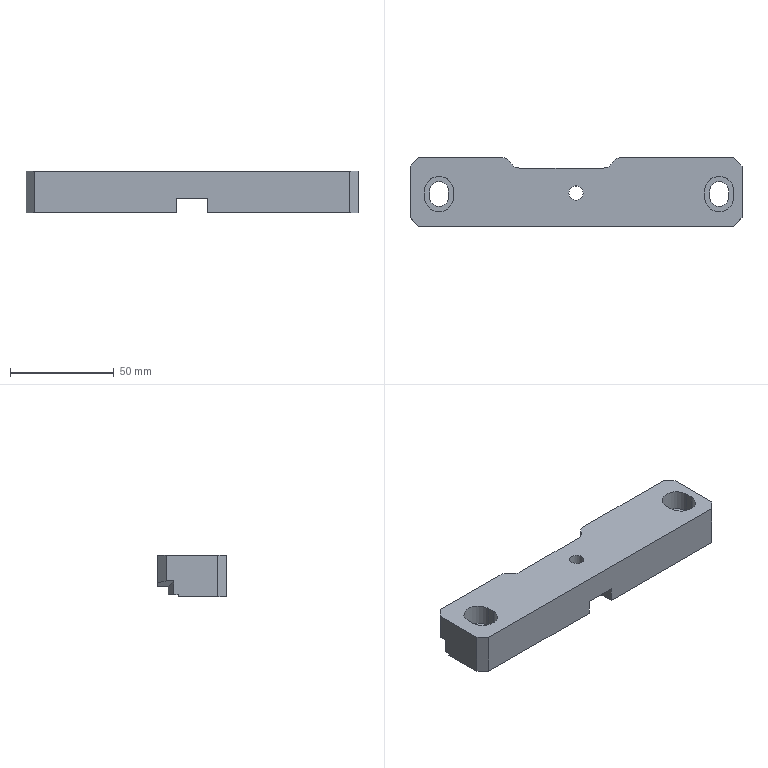Part | NX | features 20 2 | 1 solid | 49 faces | box 160 x 33 x 20 mm | volume 87274 mm3 | plane 36 | cylinder 13 | commonest cylinder face diameters 9 x4 10 x4 14 x4 6.8 x1
STEP:
#1=CARTESIAN_POINT('',(720.002,-433.5,16.5));
#2=VERTEX_POINT('',#1);
#3=CARTESIAN_POINT('',(720.002,-436.5,16.5));
#4=VERTEX_POINT('',#3);
#5=CARTESIAN_POINT('',(720.002,-450.5,16.5));
#6=DIRECTION('',(0.,-1.,0.));
#7=VECTOR('',#6,1000.);
#8=LINE('',#5,#7);
#9=EDGE_CURVE('',#2,#4,#8,.T.);
#10=ORIENTED_EDGE('',*,*,#9,.F.);
#11=CARTESIAN_POINT('',(734.002,-433.5,16.5));
#12=VERTEX_POINT('',#11);
#13=CARTESIAN_POINT('',(727.002,-433.5,16.5));
#14=DIRECTION('',(0.,0.,1.));
#15=DIRECTION('',(1.,0.,0.));
#16=AXIS2_PLACEMENT_3D('',#13,#14,#15);
#17=CIRCLE('',#16,7.);
#18=EDGE_CURVE('',#12,#2,#17,.T.);
#19=ORIENTED_EDGE('',*,*,#18,.F.);
#20=CARTESIAN_POINT('',(734.002,-436.5,16.5));
#21=VERTEX_POINT('',#20);
#22=CARTESIAN_POINT('',(734.002,-450.5,16.5));
#23=DIRECTION('',(0.,1.,0.));
#24=VECTOR('',#23,1000.);
#25=LINE('',#22,#24);
#26=EDGE_CURVE('',#21,#12,#25,.T.);
#27=ORIENTED_EDGE('',*,*,#26,.F.);
#28=CARTESIAN_POINT('',(727.002,-436.5,16.5));
#29=DIRECTION('',(0.,0.,1.));
#30=DIRECTION('',(1.,0.,0.));
#31=AXIS2_PLACEMENT_3D('',#28,#29,#30);
#32=CIRCLE('',#31,7.);
#33=EDGE_CURVE('',#4,#21,#32,.T.);
#34=ORIENTED_EDGE('',*,*,#33,.F.);
#35=EDGE_LOOP('',(#10,#19,#27,#34));
#36=FACE_BOUND('',#35,.T.);
#37=CARTESIAN_POINT('',(585.002,-433.5,16.5));
#38=VERTEX_POINT('',#37);
#39=CARTESIAN_POINT('',(585.002,-436.5,16.5));
#40=VERTEX_POINT('',#39);
#41=CARTESIAN_POINT('',(585.002,-450.5,16.5));
#42=DIRECTION('',(0.,-1.,0.));
#43=VECTOR('',#42,1000.);
#44=LINE('',#41,#43);
#45=EDGE_CURVE('',#38,#40,#44,.T.);
#46=ORIENTED_EDGE('',*,*,#45,.F.);
#47=CARTESIAN_POINT('',(599.002,-433.5,16.5));
#48=VERTEX_POINT('',#47);
#49=CARTESIAN_POINT('',(592.002,-433.5,16.5));
#50=DIRECTION('',(0.,0.,1.));
#51=DIRECTION('',(1.,0.,0.));
#52=AXIS2_PLACEMENT_3D('',#49,#50,#51);
#53=CIRCLE('',#52,7.);
#54=EDGE_CURVE('',#48,#38,#53,.T.);
#55=ORIENTED_EDGE('',*,*,#54,.F.);
#56=CARTESIAN_POINT('',(599.002,-436.5,16.5));
#57=VERTEX_POINT('',#56);
#58=CARTESIAN_POINT('',(599.002,-450.5,16.5));
#59=DIRECTION('',(0.,1.,0.));
#60=VECTOR('',#59,1000.);
#61=LINE('',#58,#60);
#62=EDGE_CURVE('',#57,#48,#61,.T.);
#63=ORIENTED_EDGE('',*,*,#62,.F.);
#64=CARTESIAN_POINT('',(592.002,-436.5,16.5));
#65=DIRECTION('',(0.,0.,1.));
#66=DIRECTION('',(1.,0.,0.));
#67=AXIS2_PLACEMENT_3D('',#64,#65,#66);
#68=CIRCLE('',#67,7.);
#69=EDGE_CURVE('',#40,#57,#68,.T.);
#70=ORIENTED_EDGE('',*,*,#69,.F.);
#71=EDGE_LOOP('',(#46,#55,#63,#70));
#72=FACE_BOUND('',#71,.T.);
#73=CARTESIAN_POINT('',(738.002,-446.5,16.5));
#74=VERTEX_POINT('',#73);
#75=CARTESIAN_POINT('',(738.002,-421.5,16.5));
#76=VERTEX_POINT('',#75);
#77=CARTESIAN_POINT('',(738.002,-450.5,16.5));
#78=DIRECTION('',(0.,1.,0.));
#79=VECTOR('',#78,1000.);
#80=LINE('',#77,#79);
#81=EDGE_CURVE('',#74,#76,#80,.T.);
#82=ORIENTED_EDGE('',*,*,#81,.T.);
#83=CARTESIAN_POINT('',(734.002,-417.5,16.5));
#84=VERTEX_POINT('',#83);
#85=CARTESIAN_POINT('',(734.002,-417.5,16.5));
#86=DIRECTION('',(-0.7071,0.7071,0.));
#87=VECTOR('',#86,1000.);
#88=LINE('',#85,#87);
#89=EDGE_CURVE('',#76,#84,#88,.T.);
#90=ORIENTED_EDGE('',*,*,#89,.T.);
#91=CARTESIAN_POINT('',(679.789,-417.5,16.5));
#92=VERTEX_POINT('',#91);
#93=CARTESIAN_POINT('',(766.002,-417.5,16.5));
#94=DIRECTION('',(-1.,0.,0.));
#95=VECTOR('',#94,1000.);
#96=LINE('',#93,#95);
#97=EDGE_CURVE('',#84,#92,#96,.T.);
#98=ORIENTED_EDGE('',*,*,#97,.T.);
#99=CARTESIAN_POINT('',(675.459,-420.,16.5));
#100=VERTEX_POINT('',#99);
#101=CARTESIAN_POINT('',(679.789,-422.5,16.5));
#102=DIRECTION('',(0.,0.,1.));
#103=DIRECTION('',(1.,0.,0.));
#104=AXIS2_PLACEMENT_3D('',#101,#102,#103);
#105=CIRCLE('',#104,5.);
#106=EDGE_CURVE('',#92,#100,#105,.T.);
#107=ORIENTED_EDGE('',*,*,#106,.T.);
#108=CARTESIAN_POINT('',(671.129,-422.5,16.5));
#109=VERTEX_POINT('',#108);
#110=CARTESIAN_POINT('',(671.129,-417.5,16.5));
#111=DIRECTION('',(0.,0.,1.));
#112=DIRECTION('',(1.,0.,0.));
#113=AXIS2_PLACEMENT_3D('',#110,#111,#112);
#114=CIRCLE('',#113,5.);
#115=EDGE_CURVE('',#109,#100,#114,.T.);
#116=ORIENTED_EDGE('',*,*,#115,.F.);
#117=CARTESIAN_POINT('',(630.929,-422.5,16.5));
#118=VERTEX_POINT('',#117);
#119=CARTESIAN_POINT('',(766.002,-422.5,16.5));
#120=DIRECTION('',(1.,0.,0.));
#121=VECTOR('',#120,1000.);
#122=LINE('',#119,#121);
#123=EDGE_CURVE('',#118,#109,#122,.T.);
#124=ORIENTED_EDGE('',*,*,#123,.F.);
#125=CARTESIAN_POINT('',(626.598,-420.,16.5));
#126=VERTEX_POINT('',#125);
#127=CARTESIAN_POINT('',(630.929,-417.5,16.5));
#128=DIRECTION('',(0.,0.,1.));
#129=DIRECTION('',(1.,0.,0.));
#130=AXIS2_PLACEMENT_3D('',#127,#128,#129);
#131=CIRCLE('',#130,5.);
#132=EDGE_CURVE('',#126,#118,#131,.T.);
#133=ORIENTED_EDGE('',*,*,#132,.F.);
#134=CARTESIAN_POINT('',(622.268,-417.5,16.5));
#135=VERTEX_POINT('',#134);
#136=CARTESIAN_POINT('',(622.268,-422.5,16.5));
#137=DIRECTION('',(0.,0.,1.));
#138=DIRECTION('',(1.,0.,0.));
#139=AXIS2_PLACEMENT_3D('',#136,#137,#138);
#140=CIRCLE('',#139,5.);
#141=EDGE_CURVE('',#126,#135,#140,.T.);
#142=ORIENTED_EDGE('',*,*,#141,.T.);
#143=CARTESIAN_POINT('',(582.002,-417.5,16.5));
#144=VERTEX_POINT('',#143);
#145=CARTESIAN_POINT('',(766.002,-417.5,16.5));
#146=DIRECTION('',(-1.,0.,0.));
#147=VECTOR('',#146,1000.);
#148=LINE('',#145,#147);
#149=EDGE_CURVE('',#135,#144,#148,.T.);
#150=ORIENTED_EDGE('',*,*,#149,.T.);
#151=CARTESIAN_POINT('',(578.002,-421.5,16.5));
#152=VERTEX_POINT('',#151);
#153=CARTESIAN_POINT('',(578.002,-421.5,16.5));
#154=DIRECTION('',(-0.7071,-0.7071,0.));
#155=VECTOR('',#154,1000.);
#156=LINE('',#153,#155);
#157=EDGE_CURVE('',#144,#152,#156,.T.);
#158=ORIENTED_EDGE('',*,*,#157,.T.);
#159=CARTESIAN_POINT('',(578.002,-446.5,16.5));
#160=VERTEX_POINT('',#159);
#161=CARTESIAN_POINT('',(578.002,-417.5,16.5));
#162=DIRECTION('',(0.,-1.,0.));
#163=VECTOR('',#162,1000.);
#164=LINE('',#161,#163);
#165=EDGE_CURVE('',#152,#160,#164,.T.);
#166=ORIENTED_EDGE('',*,*,#165,.T.);
#167=CARTESIAN_POINT('',(582.002,-450.5,16.5));
#168=VERTEX_POINT('',#167);
#169=CARTESIAN_POINT('',(582.002,-450.5,16.5));
#170=DIRECTION('',(0.7071,-0.7071,0.));
#171=VECTOR('',#170,1000.);
#172=LINE('',#169,#171);
#173=EDGE_CURVE('',#160,#168,#172,.T.);
#174=ORIENTED_EDGE('',*,*,#173,.T.);
#175=CARTESIAN_POINT('',(734.002,-450.5,16.5));
#176=VERTEX_POINT('',#175);
#177=CARTESIAN_POINT('',(686.002,-450.5,16.5));
#178=DIRECTION('',(1.,0.,0.));
#179=VECTOR('',#178,1000.);
#180=LINE('',#177,#179);
#181=EDGE_CURVE('',#168,#176,#180,.T.);
#182=ORIENTED_EDGE('',*,*,#181,.T.);
#183=CARTESIAN_POINT('',(738.002,-446.5,16.5));
#184=DIRECTION('',(0.7071,0.7071,0.));
#185=VECTOR('',#184,1000.);
#186=LINE('',#183,#185);
#187=EDGE_CURVE('',#176,#74,#186,.T.);
#188=ORIENTED_EDGE('',*,*,#187,.T.);
#189=EDGE_LOOP('',(#82,#90,#98,#107,#116,#124,#133,#142,#150,#158,#166,#174,#182,#188));
#190=FACE_BOUND('',#189,.T.);
#191=CARTESIAN_POINT('',(661.402,-434.5,16.5));
#192=VERTEX_POINT('',#191);
#193=CARTESIAN_POINT('',(658.002,-434.5,16.5));
#194=DIRECTION('',(0.,0.,-1.));
#195=DIRECTION('',(1.,0.,0.));
#196=AXIS2_PLACEMENT_3D('',#193,#194,#195);
#197=CIRCLE('',#196,3.4);
#198=EDGE_CURVE('',#192,#192,#197,.T.);
#199=ORIENTED_EDGE('',*,*,#198,.T.);
#200=EDGE_LOOP('',(#199));
#201=FACE_BOUND('',#200,.T.);
#202=CARTESIAN_POINT('',(766.002,-450.5,16.5));
#203=DIRECTION('',(0.,0.,1.));
#204=DIRECTION('',(-1.,0.,0.));
#205=AXIS2_PLACEMENT_3D('',#202,#203,#204);
#206=PLANE('',#205);
#207=ADVANCED_FACE('',(#36,#72,#190,#201),#206,.T.);
#208=CARTESIAN_POINT('',(630.929,-422.5,1.5));
#209=VERTEX_POINT('',#208);
#210=CARTESIAN_POINT('',(626.598,-420.,1.5));
#211=VERTEX_POINT('',#210);
#212=CARTESIAN_POINT('',(630.929,-417.5,1.5));
#213=DIRECTION('',(0.,0.,-1.));
#214=DIRECTION('',(-1.,0.,0.));
#215=AXIS2_PLACEMENT_3D('',#212,#213,#214);
#216=CIRCLE('',#215,5.);
#217=EDGE_CURVE('',#209,#211,#216,.T.);
#218=ORIENTED_EDGE('',*,*,#217,.F.);
#219=CARTESIAN_POINT('',(588.002,-422.5,1.5));
#220=VERTEX_POINT('',#219);
#221=CARTESIAN_POINT('',(704.001,-422.5,1.5));
#222=DIRECTION('',(1.,0.,0.));
#223=VECTOR('',#222,1000.);
#224=LINE('',#221,#223);
#225=EDGE_CURVE('',#220,#209,#224,.T.);
#226=ORIENTED_EDGE('',*,*,#225,.F.);
#227=CARTESIAN_POINT('',(588.002,-417.5,1.5));
#228=VERTEX_POINT('',#227);
#229=CARTESIAN_POINT('',(588.002,-417.5,1.5));
#230=DIRECTION('',(0.,1.,0.));
#231=VECTOR('',#230,1000.);
#232=LINE('',#229,#231);
#233=EDGE_CURVE('',#220,#228,#232,.T.);
#234=ORIENTED_EDGE('',*,*,#233,.T.);
#235=CARTESIAN_POINT('',(622.268,-417.5,1.5));
#236=VERTEX_POINT('',#235);
#237=CARTESIAN_POINT('',(714.002,-417.5,1.5));
#238=DIRECTION('',(1.,0.,0.));
#239=VECTOR('',#238,1000.);
#240=LINE('',#237,#239);
#241=EDGE_CURVE('',#228,#236,#240,.T.);
#242=ORIENTED_EDGE('',*,*,#241,.T.);
#243=CARTESIAN_POINT('',(622.268,-422.5,1.5));
#244=DIRECTION('',(0.,0.,-1.));
#245=DIRECTION('',(-1.,0.,0.));
#246=AXIS2_PLACEMENT_3D('',#243,#244,#245);
#247=CIRCLE('',#246,5.);
#248=EDGE_CURVE('',#236,#211,#247,.T.);
#249=ORIENTED_EDGE('',*,*,#248,.T.);
#250=EDGE_LOOP('',(#218,#226,#234,#242,#249));
#251=FACE_BOUND('',#250,.T.);
#252=CARTESIAN_POINT('',(736.273,-396.891,1.5));
#253=DIRECTION('',(0.,0.,-1.));
#254=DIRECTION('',(1.,0.,0.));
#255=AXIS2_PLACEMENT_3D('',#252,#253,#254);
#256=PLANE('',#255);
#257=ADVANCED_FACE('',(#251),#256,.T.);
#258=CARTESIAN_POINT('',(578.002,-427.372,-2.5));
#259=VERTEX_POINT('',#258);
#260=CARTESIAN_POINT('',(578.002,-427.372,-3.5));
#261=VERTEX_POINT('',#260);
#262=CARTESIAN_POINT('',(578.002,-427.372,11.5));
#263=DIRECTION('',(0.,0.,-1.));
#264=VECTOR('',#263,1000.);
#265=LINE('',#262,#264);
#266=EDGE_CURVE('',#259,#261,#265,.T.);
#267=ORIENTED_EDGE('',*,*,#266,.F.);
#268=CARTESIAN_POINT('',(609.502,-427.372,-2.5));
#269=VERTEX_POINT('',#268);
#270=CARTESIAN_POINT('',(684.583,-427.372,-2.5));
#271=DIRECTION('',(1.,0.,0.));
#272=VECTOR('',#271,1000.);
#273=LINE('',#270,#272);
#274=EDGE_CURVE('',#259,#269,#273,.T.);
#275=ORIENTED_EDGE('',*,*,#274,.T.);
#276=CARTESIAN_POINT('',(650.502,-427.372,-2.5));
#277=VERTEX_POINT('',#276);
#278=CARTESIAN_POINT('',(630.002,-427.372,-2.5));
#279=DIRECTION('',(1.,0.,0.));
#280=VECTOR('',#279,1000.);
#281=LINE('',#278,#280);
#282=EDGE_CURVE('',#269,#277,#281,.T.);
#283=ORIENTED_EDGE('',*,*,#282,.T.);
#284=CARTESIAN_POINT('',(650.502,-427.372,-3.5));
#285=VERTEX_POINT('',#284);
#286=CARTESIAN_POINT('',(650.502,-427.372,-9.5));
#287=DIRECTION('',(0.,0.,-1.));
#288=VECTOR('',#287,1000.);
#289=LINE('',#286,#288);
#290=EDGE_CURVE('',#277,#285,#289,.T.);
#291=ORIENTED_EDGE('',*,*,#290,.T.);
#292=CARTESIAN_POINT('',(766.002,-427.372,-3.5));
#293=DIRECTION('',(-1.,0.,0.));
#294=VECTOR('',#293,1000.);
#295=LINE('',#292,#294);
#296=EDGE_CURVE('',#285,#261,#295,.T.);
#297=ORIENTED_EDGE('',*,*,#296,.T.);
#298=EDGE_LOOP('',(#267,#275,#283,#291,#297));
#299=FACE_BOUND('',#298,.T.);
#300=CARTESIAN_POINT('',(684.583,-427.372,-21.));
#301=DIRECTION('',(0.,1.,0.));
#302=DIRECTION('',(0.,0.,-1.));
#303=AXIS2_PLACEMENT_3D('',#300,#301,#302);
#304=PLANE('',#303);
#305=ADVANCED_FACE('',(#299),#304,.T.);
#306=CARTESIAN_POINT('',(665.502,-427.372,-2.5));
#307=VERTEX_POINT('',#306);
#308=CARTESIAN_POINT('',(665.502,-427.372,-3.5));
#309=VERTEX_POINT('',#308);
#310=CARTESIAN_POINT('',(665.502,-427.372,-9.5));
#311=DIRECTION('',(0.,0.,-1.));
#312=VECTOR('',#311,1000.);
#313=LINE('',#310,#312);
#314=EDGE_CURVE('',#307,#309,#313,.T.);
#315=ORIENTED_EDGE('',*,*,#314,.F.);
#316=CARTESIAN_POINT('',(738.002,-427.372,-2.5));
#317=VERTEX_POINT('',#316);
#318=CARTESIAN_POINT('',(684.583,-427.372,-2.5));
#319=DIRECTION('',(1.,0.,0.));
#320=VECTOR('',#319,1000.);
#321=LINE('',#318,#320);
#322=EDGE_CURVE('',#307,#317,#321,.T.);
#323=ORIENTED_EDGE('',*,*,#322,.T.);
#324=CARTESIAN_POINT('',(738.002,-427.372,-3.5));
#325=VERTEX_POINT('',#324);
#326=CARTESIAN_POINT('',(738.002,-427.372,11.5));
#327=DIRECTION('',(0.,0.,1.));
#328=VECTOR('',#327,1000.);
#329=LINE('',#326,#328);
#330=EDGE_CURVE('',#325,#317,#329,.T.);
#331=ORIENTED_EDGE('',*,*,#330,.F.);
#332=CARTESIAN_POINT('',(646.002,-427.372,-3.5));
#333=DIRECTION('',(-1.,0.,0.));
#334=VECTOR('',#333,1000.);
#335=LINE('',#332,#334);
#336=EDGE_CURVE('',#325,#309,#335,.T.);
#337=ORIENTED_EDGE('',*,*,#336,.T.);
#338=EDGE_LOOP('',(#315,#323,#331,#337));
#339=FACE_BOUND('',#338,.T.);
#340=CARTESIAN_POINT('',(684.583,-427.372,-21.));
#341=DIRECTION('',(0.,1.,0.));
#342=DIRECTION('',(0.,0.,-1.));
#343=AXIS2_PLACEMENT_3D('',#340,#341,#342);
#344=PLANE('',#343);
#345=ADVANCED_FACE('',(#339),#344,.T.);
#346=CARTESIAN_POINT('',(738.002,-446.5,-3.5));
#347=VERTEX_POINT('',#346);
#348=CARTESIAN_POINT('',(734.002,-450.5,-3.5));
#349=VERTEX_POINT('',#348);
#350=CARTESIAN_POINT('',(738.002,-446.5,-3.5));
#351=DIRECTION('',(-0.7071,-0.7071,0.));
#352=VECTOR('',#351,1000.);
#353=LINE('',#350,#352);
#354=EDGE_CURVE('',#347,#349,#353,.T.);
#355=ORIENTED_EDGE('',*,*,#354,.F.);
#356=CARTESIAN_POINT('',(738.002,-446.5,11.5));
#357=DIRECTION('',(0.,0.,-1.));
#358=VECTOR('',#357,1000.);
#359=LINE('',#356,#358);
#360=EDGE_CURVE('',#74,#347,#359,.T.);
#361=ORIENTED_EDGE('',*,*,#360,.F.);
#362=ORIENTED_EDGE('',*,*,#187,.F.);
#363=CARTESIAN_POINT('',(734.002,-450.5,11.5));
#364=DIRECTION('',(0.,0.,1.));
#365=VECTOR('',#364,1000.);
#366=LINE('',#363,#365);
#367=EDGE_CURVE('',#349,#176,#366,.T.);
#368=ORIENTED_EDGE('',*,*,#367,.F.);
#369=EDGE_LOOP('',(#355,#361,#362,#368));
#370=FACE_BOUND('',#369,.T.);
#371=CARTESIAN_POINT('',(738.002,-446.5,11.5));
#372=DIRECTION('',(-0.7071,0.7071,0.));
#373=DIRECTION('',(0.,0.,-1.));
#374=AXIS2_PLACEMENT_3D('',#371,#372,#373);
#375=PLANE('',#374);
#376=ADVANCED_FACE('',(#370),#375,.F.);
#377=CARTESIAN_POINT('',(582.002,-450.5,-3.5));
#378=VERTEX_POINT('',#377);
#379=CARTESIAN_POINT('',(578.002,-446.5,-3.5));
#380=VERTEX_POINT('',#379);
#381=CARTESIAN_POINT('',(582.002,-450.5,-3.5));
#382=DIRECTION('',(-0.7071,0.7071,0.));
#383=VECTOR('',#382,1000.);
#384=LINE('',#381,#383);
#385=EDGE_CURVE('',#378,#380,#384,.T.);
#386=ORIENTED_EDGE('',*,*,#385,.F.);
#387=CARTESIAN_POINT('',(582.002,-450.5,11.5));
#388=DIRECTION('',(0.,0.,-1.));
#389=VECTOR('',#388,1000.);
#390=LINE('',#387,#389);
#391=EDGE_CURVE('',#168,#378,#390,.T.);
#392=ORIENTED_EDGE('',*,*,#391,.F.);
#393=ORIENTED_EDGE('',*,*,#173,.F.);
#394=CARTESIAN_POINT('',(578.002,-446.5,11.5));
#395=DIRECTION('',(0.,0.,1.));
#396=VECTOR('',#395,1000.);
#397=LINE('',#394,#396);
#398=EDGE_CURVE('',#380,#160,#397,.T.);
#399=ORIENTED_EDGE('',*,*,#398,.F.);
#400=EDGE_LOOP('',(#386,#392,#393,#399));
#401=FACE_BOUND('',#400,.T.);
#402=CARTESIAN_POINT('',(582.002,-450.5,11.5));
#403=DIRECTION('',(0.7071,0.7071,0.));
#404=DIRECTION('',(0.,0.,-1.));
#405=AXIS2_PLACEMENT_3D('',#402,#403,#404);
#406=PLANE('',#405);
#407=ADVANCED_FACE('',(#401),#406,.F.);
#408=ORIENTED_EDGE('',*,*,#33,.T.);
#409=CARTESIAN_POINT('',(734.002,-436.5,6.5));
#410=VERTEX_POINT('',#409);
#411=CARTESIAN_POINT('',(734.002,-436.5,42.5));
#412=DIRECTION('',(0.,0.,1.));
#413=VECTOR('',#412,1000.);
#414=LINE('',#411,#413);
#415=EDGE_CURVE('',#410,#21,#414,.T.);
#416=ORIENTED_EDGE('',*,*,#415,.F.);
#417=CARTESIAN_POINT('',(720.002,-436.5,6.5));
#418=VERTEX_POINT('',#417);
#419=CARTESIAN_POINT('',(727.002,-436.5,6.5));
#420=DIRECTION('',(0.,0.,1.));
#421=DIRECTION('',(-1.,0.,0.));
#422=AXIS2_PLACEMENT_3D('',#419,#420,#421);
#423=CIRCLE('',#422,7.);
#424=EDGE_CURVE('',#418,#410,#423,.T.);
#425=ORIENTED_EDGE('',*,*,#424,.F.);
#426=CARTESIAN_POINT('',(720.002,-436.5,42.5));
#427=DIRECTION('',(0.,0.,1.));
#428=VECTOR('',#427,1000.);
#429=LINE('',#426,#428);
#430=EDGE_CURVE('',#418,#4,#429,.T.);
#431=ORIENTED_EDGE('',*,*,#430,.T.);
#432=EDGE_LOOP('',(#408,#416,#425,#431));
#433=FACE_BOUND('',#432,.T.);
#434=CARTESIAN_POINT('',(727.002,-436.5,42.5));
#435=DIRECTION('',(0.,0.,-1.));
#436=DIRECTION('',(1.,0.,0.));
#437=AXIS2_PLACEMENT_3D('',#434,#435,#436);
#438=CYLINDRICAL_SURFACE('',#437,7.);
#439=ADVANCED_FACE('',(#433),#438,.F.);
#440=CARTESIAN_POINT('',(731.502,-436.5,6.5));
#441=VERTEX_POINT('',#440);
#442=CARTESIAN_POINT('',(722.502,-436.5,6.5));
#443=VERTEX_POINT('',#442);
#444=CARTESIAN_POINT('',(727.002,-436.5,6.5));
#445=DIRECTION('',(0.,0.,-1.));
#446=DIRECTION('',(-1.,0.,0.));
#447=AXIS2_PLACEMENT_3D('',#444,#445,#446);
#448=CIRCLE('',#447,4.5);
#449=EDGE_CURVE('',#441,#443,#448,.T.);
#450=ORIENTED_EDGE('',*,*,#449,.F.);
#451=CARTESIAN_POINT('',(731.502,-436.5,-3.5));
#452=VERTEX_POINT('',#451);
#453=CARTESIAN_POINT('',(731.502,-436.5,42.5));
#454=DIRECTION('',(0.,0.,1.));
#455=VECTOR('',#454,1000.);
#456=LINE('',#453,#455);
#457=EDGE_CURVE('',#452,#441,#456,.T.);
#458=ORIENTED_EDGE('',*,*,#457,.F.);
#459=CARTESIAN_POINT('',(722.502,-436.5,-3.5));
#460=VERTEX_POINT('',#459);
#461=CARTESIAN_POINT('',(727.002,-436.5,-3.5));
#462=DIRECTION('',(0.,0.,1.));
#463=DIRECTION('',(1.,0.,0.));
#464=AXIS2_PLACEMENT_3D('',#461,#462,#463);
#465=CIRCLE('',#464,4.5);
#466=EDGE_CURVE('',#460,#452,#465,.T.);
#467=ORIENTED_EDGE('',*,*,#466,.F.);
#468=CARTESIAN_POINT('',(722.502,-436.5,42.5));
#469=DIRECTION('',(0.,0.,1.));
#470=VECTOR('',#469,1000.);
#471=LINE('',#468,#470);
#472=EDGE_CURVE('',#460,#443,#471,.T.);
#473=ORIENTED_EDGE('',*,*,#472,.T.);
#474=EDGE_LOOP('',(#450,#458,#467,#473));
#475=FACE_BOUND('',#474,.T.);
#476=CARTESIAN_POINT('',(727.002,-436.5,42.5));
#477=DIRECTION('',(0.,0.,-1.));
#478=DIRECTION('',(1.,0.,0.));
#479=AXIS2_PLACEMENT_3D('',#476,#477,#478);
#480=CYLINDRICAL_SURFACE('',#479,4.5);
#481=ADVANCED_FACE('',(#475),#480,.F.);
#482=CARTESIAN_POINT('',(731.502,-433.5,6.5));
#483=VERTEX_POINT('',#482);
#484=CARTESIAN_POINT('',(731.502,-439.5,6.5));
#485=DIRECTION('',(0.,-1.,0.));
#486=VECTOR('',#485,1000.);
#487=LINE('',#484,#486);
#488=EDGE_CURVE('',#483,#441,#487,.T.);
#489=ORIENTED_EDGE('',*,*,#488,.F.);
#490=CARTESIAN_POINT('',(731.502,-433.5,-3.5));
#491=VERTEX_POINT('',#490);
#492=CARTESIAN_POINT('',(731.502,-433.5,42.5));
#493=DIRECTION('',(0.,0.,1.));
#494=VECTOR('',#493,1000.);
#495=LINE('',#492,#494);
#496=EDGE_CURVE('',#491,#483,#495,.T.);
#497=ORIENTED_EDGE('',*,*,#496,.F.);
#498=CARTESIAN_POINT('',(731.502,-439.5,-3.5));
#499=DIRECTION('',(0.,1.,0.));
#500=VECTOR('',#499,1000.);
#501=LINE('',#498,#500);
#502=EDGE_CURVE('',#452,#491,#501,.T.);
#503=ORIENTED_EDGE('',*,*,#502,.F.);
#504=ORIENTED_EDGE('',*,*,#457,.T.);
#505=EDGE_LOOP('',(#489,#497,#503,#504));
#506=FACE_BOUND('',#505,.T.);
#507=CARTESIAN_POINT('',(731.502,-439.5,42.5));
#508=DIRECTION('',(-1.,0.,0.));
#509=DIRECTION('',(0.,0.,-1.));
#510=AXIS2_PLACEMENT_3D('',#507,#508,#509);
#511=PLANE('',#510);
#512=ADVANCED_FACE('',(#506),#511,.T.);
#513=CARTESIAN_POINT('',(722.502,-433.5,6.5));
#514=VERTEX_POINT('',#513);
#515=CARTESIAN_POINT('',(727.002,-433.5,6.5));
#516=DIRECTION('',(0.,0.,-1.));
#517=DIRECTION('',(-1.,0.,0.));
#518=AXIS2_PLACEMENT_3D('',#515,#516,#517);
#519=CIRCLE('',#518,4.5);
#520=EDGE_CURVE('',#514,#483,#519,.T.);
#521=ORIENTED_EDGE('',*,*,#520,.F.);
#522=CARTESIAN_POINT('',(722.502,-433.5,-3.5));
#523=VERTEX_POINT('',#522);
#524=CARTESIAN_POINT('',(722.502,-433.5,42.5));
#525=DIRECTION('',(0.,0.,1.));
#526=VECTOR('',#525,1000.);
#527=LINE('',#524,#526);
#528=EDGE_CURVE('',#523,#514,#527,.T.);
#529=ORIENTED_EDGE('',*,*,#528,.F.);
#530=CARTESIAN_POINT('',(727.002,-433.5,-3.5));
#531=DIRECTION('',(0.,0.,1.));
#532=DIRECTION('',(1.,0.,0.));
#533=AXIS2_PLACEMENT_3D('',#530,#531,#532);
#534=CIRCLE('',#533,4.5);
#535=EDGE_CURVE('',#491,#523,#534,.T.);
#536=ORIENTED_EDGE('',*,*,#535,.F.);
#537=ORIENTED_EDGE('',*,*,#496,.T.);
#538=EDGE_LOOP('',(#521,#529,#536,#537));
#539=FACE_BOUND('',#538,.T.);
#540=CARTESIAN_POINT('',(727.002,-433.5,42.5));
#541=DIRECTION('',(0.,0.,-1.));
#542=DIRECTION('',(1.,0.,0.));
#543=AXIS2_PLACEMENT_3D('',#540,#541,#542);
#544=CYLINDRICAL_SURFACE('',#543,4.5);
#545=ADVANCED_FACE('',(#539),#544,.F.);
#546=CARTESIAN_POINT('',(722.502,-432.5,6.5));
#547=DIRECTION('',(0.,1.,0.));
#548=VECTOR('',#547,1000.);
#549=LINE('',#546,#548);
#550=EDGE_CURVE('',#443,#514,#549,.T.);
#551=ORIENTED_EDGE('',*,*,#550,.F.);
#552=ORIENTED_EDGE('',*,*,#472,.F.);
#553=CARTESIAN_POINT('',(722.502,-432.5,-3.5));
#554=DIRECTION('',(0.,-1.,0.));
#555=VECTOR('',#554,1000.);
#556=LINE('',#553,#555);
#557=EDGE_CURVE('',#523,#460,#556,.T.);
#558=ORIENTED_EDGE('',*,*,#557,.F.);
#559=ORIENTED_EDGE('',*,*,#528,.T.);
#560=EDGE_LOOP('',(#551,#552,#558,#559));
#561=FACE_BOUND('',#560,.T.);
#562=CARTESIAN_POINT('',(722.502,-432.5,42.5));
#563=DIRECTION('',(1.,0.,0.));
#564=DIRECTION('',(0.,0.,1.));
#565=AXIS2_PLACEMENT_3D('',#562,#563,#564);
#566=PLANE('',#565);
#567=ADVANCED_FACE('',(#561),#566,.T.);
#568=ORIENTED_EDGE('',*,*,#69,.T.);
#569=CARTESIAN_POINT('',(599.002,-436.5,6.5));
#570=VERTEX_POINT('',#569);
#571=CARTESIAN_POINT('',(599.002,-436.5,42.5));
#572=DIRECTION('',(0.,0.,-1.));
#573=VECTOR('',#572,1000.);
#574=LINE('',#571,#573);
#575=EDGE_CURVE('',#57,#570,#574,.T.);
#576=ORIENTED_EDGE('',*,*,#575,.T.);
#577=CARTESIAN_POINT('',(585.002,-436.5,6.5));
#578=VERTEX_POINT('',#577);
#579=CARTESIAN_POINT('',(592.002,-436.5,6.5));
#580=DIRECTION('',(0.,0.,1.));
#581=DIRECTION('',(-1.,0.,0.));
#582=AXIS2_PLACEMENT_3D('',#579,#580,#581);
#583=CIRCLE('',#582,7.);
#584=EDGE_CURVE('',#578,#570,#583,.T.);
#585=ORIENTED_EDGE('',*,*,#584,.F.);
#586=CARTESIAN_POINT('',(585.002,-436.5,42.5));
#587=DIRECTION('',(0.,0.,-1.));
#588=VECTOR('',#587,1000.);
#589=LINE('',#586,#588);
#590=EDGE_CURVE('',#40,#578,#589,.T.);
#591=ORIENTED_EDGE('',*,*,#590,.F.);
#592=EDGE_LOOP('',(#568,#576,#585,#591));
#593=FACE_BOUND('',#592,.T.);
#594=CARTESIAN_POINT('',(592.002,-436.5,42.5));
#595=DIRECTION('',(0.,0.,-1.));
#596=DIRECTION('',(-1.,0.,0.));
#597=AXIS2_PLACEMENT_3D('',#594,#595,#596);
#598=CYLINDRICAL_SURFACE('',#597,7.);
#599=ADVANCED_FACE('',(#593),#598,.F.);
#600=CARTESIAN_POINT('',(587.502,-433.5,6.5));
#601=VERTEX_POINT('',#600);
#602=CARTESIAN_POINT('',(596.502,-433.5,6.5));
#603=VERTEX_POINT('',#602);
#604=CARTESIAN_POINT('',(592.002,-433.5,6.5));
#605=DIRECTION('',(0.,0.,-1.));
#606=DIRECTION('',(-1.,0.,0.));
#607=AXIS2_PLACEMENT_3D('',#604,#605,#606);
#608=CIRCLE('',#607,4.5);
#609=EDGE_CURVE('',#601,#603,#608,.T.);
#610=ORIENTED_EDGE('',*,*,#609,.F.);
#611=CARTESIAN_POINT('',(587.502,-433.5,-3.5));
#612=VERTEX_POINT('',#611);
#613=CARTESIAN_POINT('',(587.502,-433.5,42.5));
#614=DIRECTION('',(0.,0.,-1.));
#615=VECTOR('',#614,1000.);
#616=LINE('',#613,#615);
#617=EDGE_CURVE('',#601,#612,#616,.T.);
#618=ORIENTED_EDGE('',*,*,#617,.T.);
#619=CARTESIAN_POINT('',(596.502,-433.5,-3.5));
#620=VERTEX_POINT('',#619);
#621=CARTESIAN_POINT('',(592.002,-433.5,-3.5));
#622=DIRECTION('',(0.,0.,-1.));
#623=DIRECTION('',(1.,0.,0.));
#624=AXIS2_PLACEMENT_3D('',#621,#622,#623);
#625=CIRCLE('',#624,4.5);
#626=EDGE_CURVE('',#612,#620,#625,.T.);
#627=ORIENTED_EDGE('',*,*,#626,.T.);
#628=CARTESIAN_POINT('',(596.502,-433.5,42.5));
#629=DIRECTION('',(0.,0.,-1.));
#630=VECTOR('',#629,1000.);
#631=LINE('',#628,#630);
#632=EDGE_CURVE('',#603,#620,#631,.T.);
#633=ORIENTED_EDGE('',*,*,#632,.F.);
#634=EDGE_LOOP('',(#610,#618,#627,#633));
#635=FACE_BOUND('',#634,.T.);
#636=CARTESIAN_POINT('',(592.002,-433.5,42.5));
#637=DIRECTION('',(0.,0.,-1.));
#638=DIRECTION('',(-1.,0.,0.));
#639=AXIS2_PLACEMENT_3D('',#636,#637,#638);
#640=CYLINDRICAL_SURFACE('',#639,4.5);
#641=ADVANCED_FACE('',(#635),#640,.F.);
#642=CARTESIAN_POINT('',(587.502,-436.5,6.5));
#643=VERTEX_POINT('',#642);
#644=CARTESIAN_POINT('',(587.502,-439.5,6.5));
#645=DIRECTION('',(0.,1.,0.));
#646=VECTOR('',#645,1000.);
#647=LINE('',#644,#646);
#648=EDGE_CURVE('',#643,#601,#647,.T.);
#649=ORIENTED_EDGE('',*,*,#648,.F.);
#650=CARTESIAN_POINT('',(587.502,-436.5,-3.5));
#651=VERTEX_POINT('',#650);
#652=CARTESIAN_POINT('',(587.502,-436.5,42.5));
#653=DIRECTION('',(0.,0.,-1.));
#654=VECTOR('',#653,1000.);
#655=LINE('',#652,#654);
#656=EDGE_CURVE('',#643,#651,#655,.T.);
#657=ORIENTED_EDGE('',*,*,#656,.T.);
#658=CARTESIAN_POINT('',(587.502,-450.5,-3.5));
#659=DIRECTION('',(0.,1.,0.));
#660=VECTOR('',#659,1000.);
#661=LINE('',#658,#660);
#662=EDGE_CURVE('',#651,#612,#661,.T.);
#663=ORIENTED_EDGE('',*,*,#662,.T.);
#664=ORIENTED_EDGE('',*,*,#617,.F.);
#665=EDGE_LOOP('',(#649,#657,#663,#664));
#666=FACE_BOUND('',#665,.T.);
#667=CARTESIAN_POINT('',(587.502,-439.5,42.5));
#668=DIRECTION('',(1.,0.,0.));
#669=DIRECTION('',(0.,0.,-1.));
#670=AXIS2_PLACEMENT_3D('',#667,#668,#669);
#671=PLANE('',#670);
#672=ADVANCED_FACE('',(#666),#671,.T.);
#673=CARTESIAN_POINT('',(596.502,-436.5,6.5));
#674=VERTEX_POINT('',#673);
#675=CARTESIAN_POINT('',(592.002,-436.5,6.5));
#676=DIRECTION('',(0.,0.,-1.));
#677=DIRECTION('',(-1.,0.,0.));
#678=AXIS2_PLACEMENT_3D('',#675,#676,#677);
#679=CIRCLE('',#678,4.5);
#680=EDGE_CURVE('',#674,#643,#679,.T.);
#681=ORIENTED_EDGE('',*,*,#680,.F.);
#682=CARTESIAN_POINT('',(596.502,-436.5,-3.5));
#683=VERTEX_POINT('',#682);
#684=CARTESIAN_POINT('',(596.502,-436.5,42.5));
#685=DIRECTION('',(0.,0.,-1.));
#686=VECTOR('',#685,1000.);
#687=LINE('',#684,#686);
#688=EDGE_CURVE('',#674,#683,#687,.T.);
#689=ORIENTED_EDGE('',*,*,#688,.T.);
#690=CARTESIAN_POINT('',(592.002,-436.5,-3.5));
#691=DIRECTION('',(0.,0.,-1.));
#692=DIRECTION('',(1.,0.,0.));
#693=AXIS2_PLACEMENT_3D('',#690,#691,#692);
#694=CIRCLE('',#693,4.5);
#695=EDGE_CURVE('',#683,#651,#694,.T.);
#696=ORIENTED_EDGE('',*,*,#695,.T.);
#697=ORIENTED_EDGE('',*,*,#656,.F.);
#698=EDGE_LOOP('',(#681,#689,#696,#697));
#699=FACE_BOUND('',#698,.T.);
#700=CARTESIAN_POINT('',(592.002,-436.5,42.5));
#701=DIRECTION('',(0.,0.,-1.));
#702=DIRECTION('',(-1.,0.,0.));
#703=AXIS2_PLACEMENT_3D('',#700,#701,#702);
#704=CYLINDRICAL_SURFACE('',#703,4.5);
#705=ADVANCED_FACE('',(#699),#704,.F.);
#706=CARTESIAN_POINT('',(596.502,-432.5,6.5));
#707=DIRECTION('',(0.,-1.,0.));
#708=VECTOR('',#707,1000.);
#709=LINE('',#706,#708);
#710=EDGE_CURVE('',#603,#674,#709,.T.);
#711=ORIENTED_EDGE('',*,*,#710,.F.);
#712=ORIENTED_EDGE('',*,*,#632,.T.);
#713=CARTESIAN_POINT('',(596.502,-450.5,-3.5));
#714=DIRECTION('',(0.,-1.,0.));
#715=VECTOR('',#714,1000.);
#716=LINE('',#713,#715);
#717=EDGE_CURVE('',#620,#683,#716,.T.);
#718=ORIENTED_EDGE('',*,*,#717,.T.);
#719=ORIENTED_EDGE('',*,*,#688,.F.);
#720=EDGE_LOOP('',(#711,#712,#718,#719));
#721=FACE_BOUND('',#720,.T.);
#722=CARTESIAN_POINT('',(596.502,-432.5,42.5));
#723=DIRECTION('',(-1.,0.,0.));
#724=DIRECTION('',(0.,0.,1.));
#725=AXIS2_PLACEMENT_3D('',#722,#723,#724);
#726=PLANE('',#725);
#727=ADVANCED_FACE('',(#721),#726,.T.);
#728=ORIENTED_EDGE('',*,*,#26,.T.);
#729=CARTESIAN_POINT('',(734.002,-433.5,6.5));
#730=VERTEX_POINT('',#729);
#731=CARTESIAN_POINT('',(734.002,-433.5,42.5));
#732=DIRECTION('',(0.,0.,1.));
#733=VECTOR('',#732,1000.);
#734=LINE('',#731,#733);
#735=EDGE_CURVE('',#730,#12,#734,.T.);
#736=ORIENTED_EDGE('',*,*,#735,.F.);
#737=CARTESIAN_POINT('',(734.002,-432.5,6.5));
#738=DIRECTION('',(0.,1.,0.));
#739=VECTOR('',#738,1000.);
#740=LINE('',#737,#739);
#741=EDGE_CURVE('',#410,#730,#740,.T.);
#742=ORIENTED_EDGE('',*,*,#741,.F.);
#743=ORIENTED_EDGE('',*,*,#415,.T.);
#744=EDGE_LOOP('',(#728,#736,#742,#743));
#745=FACE_BOUND('',#744,.T.);
#746=CARTESIAN_POINT('',(734.002,-432.5,42.5));
#747=DIRECTION('',(1.,0.,0.));
#748=DIRECTION('',(0.,0.,1.));
#749=AXIS2_PLACEMENT_3D('',#746,#747,#748);
#750=PLANE('',#749);
#751=ADVANCED_FACE('',(#745),#750,.F.);
#752=ORIENTED_EDGE('',*,*,#9,.T.);
#753=ORIENTED_EDGE('',*,*,#430,.F.);
#754=CARTESIAN_POINT('',(720.002,-433.5,6.5));
#755=VERTEX_POINT('',#754);
#756=CARTESIAN_POINT('',(720.002,-439.5,6.5));
#757=DIRECTION('',(0.,-1.,0.));
#758=VECTOR('',#757,1000.);
#759=LINE('',#756,#758);
#760=EDGE_CURVE('',#755,#418,#759,.T.);
#761=ORIENTED_EDGE('',*,*,#760,.F.);
#762=CARTESIAN_POINT('',(720.002,-433.5,42.5));
#763=DIRECTION('',(0.,0.,1.));
#764=VECTOR('',#763,1000.);
#765=LINE('',#762,#764);
#766=EDGE_CURVE('',#755,#2,#765,.T.);
#767=ORIENTED_EDGE('',*,*,#766,.T.);
#768=EDGE_LOOP('',(#752,#753,#761,#767));
#769=FACE_BOUND('',#768,.T.);
#770=CARTESIAN_POINT('',(720.002,-439.5,42.5));
#771=DIRECTION('',(-1.,0.,0.));
#772=DIRECTION('',(0.,0.,-1.));
#773=AXIS2_PLACEMENT_3D('',#770,#771,#772);
#774=PLANE('',#773);
#775=ADVANCED_FACE('',(#769),#774,.F.);
#776=ORIENTED_EDGE('',*,*,#62,.T.);
#777=CARTESIAN_POINT('',(599.002,-433.5,6.5));
#778=VERTEX_POINT('',#777);
#779=CARTESIAN_POINT('',(599.002,-433.5,42.5));
#780=DIRECTION('',(0.,0.,-1.));
#781=VECTOR('',#780,1000.);
#782=LINE('',#779,#781);
#783=EDGE_CURVE('',#48,#778,#782,.T.);
#784=ORIENTED_EDGE('',*,*,#783,.T.);
#785=CARTESIAN_POINT('',(599.002,-439.5,6.5));
#786=DIRECTION('',(0.,1.,0.));
#787=VECTOR('',#786,1000.);
#788=LINE('',#785,#787);
#789=EDGE_CURVE('',#570,#778,#788,.T.);
#790=ORIENTED_EDGE('',*,*,#789,.F.);
#791=ORIENTED_EDGE('',*,*,#575,.F.);
#792=EDGE_LOOP('',(#776,#784,#790,#791));
#793=FACE_BOUND('',#792,.T.);
#794=CARTESIAN_POINT('',(599.002,-439.5,42.5));
#795=DIRECTION('',(1.,0.,0.));
#796=DIRECTION('',(0.,0.,-1.));
#797=AXIS2_PLACEMENT_3D('',#794,#795,#796);
#798=PLANE('',#797);
#799=ADVANCED_FACE('',(#793),#798,.F.);
#800=ORIENTED_EDGE('',*,*,#45,.T.);
#801=ORIENTED_EDGE('',*,*,#590,.T.);
#802=CARTESIAN_POINT('',(585.002,-433.5,6.5));
#803=VERTEX_POINT('',#802);
#804=CARTESIAN_POINT('',(585.002,-432.5,6.5));
#805=DIRECTION('',(0.,-1.,0.));
#806=VECTOR('',#805,1000.);
#807=LINE('',#804,#806);
#808=EDGE_CURVE('',#803,#578,#807,.T.);
#809=ORIENTED_EDGE('',*,*,#808,.F.);
#810=CARTESIAN_POINT('',(585.002,-433.5,42.5));
#811=DIRECTION('',(0.,0.,-1.));
#812=VECTOR('',#811,1000.);
#813=LINE('',#810,#812);
#814=EDGE_CURVE('',#38,#803,#813,.T.);
#815=ORIENTED_EDGE('',*,*,#814,.F.);
#816=EDGE_LOOP('',(#800,#801,#809,#815));
#817=FACE_BOUND('',#816,.T.);
#818=CARTESIAN_POINT('',(585.002,-432.5,42.5));
#819=DIRECTION('',(-1.,0.,0.));
#820=DIRECTION('',(0.,0.,1.));
#821=AXIS2_PLACEMENT_3D('',#818,#819,#820);
#822=PLANE('',#821);
#823=ADVANCED_FACE('',(#817),#822,.F.);
#824=CARTESIAN_POINT('',(650.502,-450.5,-3.5));
#825=VERTEX_POINT('',#824);
#826=CARTESIAN_POINT('',(650.502,-450.5,3.5));
#827=VERTEX_POINT('',#826);
#828=CARTESIAN_POINT('',(650.502,-450.5,11.5));
#829=DIRECTION('',(0.,0.,1.));
#830=VECTOR('',#829,1000.);
#831=LINE('',#828,#830);
#832=EDGE_CURVE('',#825,#827,#831,.T.);
#833=ORIENTED_EDGE('',*,*,#832,.T.);
#834=CARTESIAN_POINT('',(665.502,-450.5,3.5));
#835=VERTEX_POINT('',#834);
#836=CARTESIAN_POINT('',(686.002,-450.5,3.5));
#837=DIRECTION('',(1.,0.,0.));
#838=VECTOR('',#837,1000.);
#839=LINE('',#836,#838);
#840=EDGE_CURVE('',#827,#835,#839,.T.);
#841=ORIENTED_EDGE('',*,*,#840,.T.);
#842=CARTESIAN_POINT('',(665.502,-450.5,-3.5));
#843=VERTEX_POINT('',#842);
#844=CARTESIAN_POINT('',(665.502,-450.5,11.5));
#845=DIRECTION('',(0.,0.,-1.));
#846=VECTOR('',#845,1000.);
#847=LINE('',#844,#846);
#848=EDGE_CURVE('',#835,#843,#847,.T.);
#849=ORIENTED_EDGE('',*,*,#848,.T.);
#850=CARTESIAN_POINT('',(696.002,-450.5,-3.5));
#851=DIRECTION('',(1.,0.,0.));
#852=VECTOR('',#851,1000.);
#853=LINE('',#850,#852);
#854=EDGE_CURVE('',#843,#349,#853,.T.);
#855=ORIENTED_EDGE('',*,*,#854,.T.);
#856=ORIENTED_EDGE('',*,*,#367,.T.);
#857=ORIENTED_EDGE('',*,*,#181,.F.);
#858=ORIENTED_EDGE('',*,*,#391,.T.);
#859=CARTESIAN_POINT('',(696.002,-450.5,-3.5));
#860=DIRECTION('',(1.,0.,0.));
#861=VECTOR('',#860,1000.);
#862=LINE('',#859,#861);
#863=EDGE_CURVE('',#378,#825,#862,.T.);
#864=ORIENTED_EDGE('',*,*,#863,.T.);
#865=EDGE_LOOP('',(#833,#841,#849,#855,#856,#857,#858,#864));
#866=FACE_BOUND('',#865,.T.);
#867=CARTESIAN_POINT('',(686.002,-450.5,11.5));
#868=DIRECTION('',(0.,1.,0.));
#869=DIRECTION('',(0.,0.,-1.));
#870=AXIS2_PLACEMENT_3D('',#867,#868,#869);
#871=PLANE('',#870);
#872=ADVANCED_FACE('',(#866),#871,.F.);
#873=ORIENTED_EDGE('',*,*,#165,.F.);
#874=CARTESIAN_POINT('',(578.002,-421.5,4.179));
#875=VERTEX_POINT('',#874);
#876=CARTESIAN_POINT('',(578.002,-421.5,11.5));
#877=DIRECTION('',(0.,0.,-1.));
#878=VECTOR('',#877,1000.);
#879=LINE('',#876,#878);
#880=EDGE_CURVE('',#152,#875,#879,.T.);
#881=ORIENTED_EDGE('',*,*,#880,.T.);
#882=CARTESIAN_POINT('',(578.002,-425.179,4.179));
#883=VERTEX_POINT('',#882);
#884=CARTESIAN_POINT('',(578.002,-425.179,4.179));
#885=DIRECTION('',(0.,-1.,0.));
#886=VECTOR('',#885,1000.);
#887=LINE('',#884,#886);
#888=EDGE_CURVE('',#875,#883,#887,.T.);
#889=ORIENTED_EDGE('',*,*,#888,.T.);
#890=CARTESIAN_POINT('',(578.002,-425.179,-2.5));
#891=VERTEX_POINT('',#890);
#892=CARTESIAN_POINT('',(578.002,-425.179,3.5));
#893=DIRECTION('',(0.,0.,-1.));
#894=VECTOR('',#893,1000.);
#895=LINE('',#892,#894);
#896=EDGE_CURVE('',#883,#891,#895,.T.);
#897=ORIENTED_EDGE('',*,*,#896,.T.);
#898=CARTESIAN_POINT('',(578.002,-417.5,-2.5));
#899=DIRECTION('',(0.,-1.,0.));
#900=VECTOR('',#899,1000.);
#901=LINE('',#898,#900);
#902=EDGE_CURVE('',#891,#259,#901,.T.);
#903=ORIENTED_EDGE('',*,*,#902,.T.);
#904=ORIENTED_EDGE('',*,*,#266,.T.);
#905=CARTESIAN_POINT('',(578.002,-417.5,-3.5));
#906=DIRECTION('',(0.,-1.,0.));
#907=VECTOR('',#906,1000.);
#908=LINE('',#905,#907);
#909=EDGE_CURVE('',#261,#380,#908,.T.);
#910=ORIENTED_EDGE('',*,*,#909,.T.);
#911=ORIENTED_EDGE('',*,*,#398,.T.);
#912=EDGE_LOOP('',(#873,#881,#889,#897,#903,#904,#910,#911));
#913=FACE_BOUND('',#912,.T.);
#914=CARTESIAN_POINT('',(578.002,-417.5,11.5));
#915=DIRECTION('',(1.,0.,0.));
#916=DIRECTION('',(0.,0.,1.));
#917=AXIS2_PLACEMENT_3D('',#914,#915,#916);
#918=PLANE('',#917);
#919=ADVANCED_FACE('',(#913),#918,.F.);
#920=CARTESIAN_POINT('',(661.402,-434.5,3.5));
#921=VERTEX_POINT('',#920);
#922=CARTESIAN_POINT('',(658.002,-434.5,3.5));
#923=DIRECTION('',(0.,0.,1.));
#924=DIRECTION('',(1.,0.,0.));
#925=AXIS2_PLACEMENT_3D('',#922,#923,#924);
#926=CIRCLE('',#925,3.4);
#927=EDGE_CURVE('',#921,#921,#926,.T.);
#928=ORIENTED_EDGE('',*,*,#927,.T.);
#929=EDGE_LOOP('',(#928));
#930=FACE_BOUND('',#929,.T.);
#931=ORIENTED_EDGE('',*,*,#840,.F.);
#932=CARTESIAN_POINT('',(650.502,-422.5,3.5));
#933=VERTEX_POINT('',#932);
#934=CARTESIAN_POINT('',(650.502,-436.5,3.5));
#935=DIRECTION('',(0.,1.,0.));
#936=VECTOR('',#935,1000.);
#937=LINE('',#934,#936);
#938=EDGE_CURVE('',#827,#933,#937,.T.);
#939=ORIENTED_EDGE('',*,*,#938,.T.);
#940=CARTESIAN_POINT('',(665.502,-422.5,3.5));
#941=VERTEX_POINT('',#940);
#942=CARTESIAN_POINT('',(704.001,-422.5,3.5));
#943=DIRECTION('',(-1.,0.,0.));
#944=VECTOR('',#943,1000.);
#945=LINE('',#942,#944);
#946=EDGE_CURVE('',#941,#933,#945,.T.);
#947=ORIENTED_EDGE('',*,*,#946,.F.);
#948=CARTESIAN_POINT('',(665.502,-436.5,3.5));
#949=DIRECTION('',(0.,1.,0.));
#950=VECTOR('',#949,1000.);
#951=LINE('',#948,#950);
#952=EDGE_CURVE('',#835,#941,#951,.T.);
#953=ORIENTED_EDGE('',*,*,#952,.F.);
#954=EDGE_LOOP('',(#931,#939,#947,#953));
#955=FACE_BOUND('',#954,.T.);
#956=CARTESIAN_POINT('',(617.002,-436.5,3.5));
#957=DIRECTION('',(0.,0.,1.));
#958=DIRECTION('',(0.,-1.,0.));
#959=AXIS2_PLACEMENT_3D('',#956,#957,#958);
#960=PLANE('',#959);
#961=ADVANCED_FACE('',(#930,#955),#960,.F.);
#962=ORIENTED_EDGE('',*,*,#717,.F.);
#963=ORIENTED_EDGE('',*,*,#626,.F.);
#964=ORIENTED_EDGE('',*,*,#662,.F.);
#965=ORIENTED_EDGE('',*,*,#695,.F.);
#966=EDGE_LOOP('',(#962,#963,#964,#965));
#967=FACE_BOUND('',#966,.T.);
#968=ORIENTED_EDGE('',*,*,#296,.F.);
#969=CARTESIAN_POINT('',(650.502,-450.5,-3.5));
#970=DIRECTION('',(0.,-1.,0.));
#971=VECTOR('',#970,1000.);
#972=LINE('',#969,#971);
#973=EDGE_CURVE('',#285,#825,#972,.T.);
#974=ORIENTED_EDGE('',*,*,#973,.T.);
#975=ORIENTED_EDGE('',*,*,#863,.F.);
#976=ORIENTED_EDGE('',*,*,#385,.T.);
#977=ORIENTED_EDGE('',*,*,#909,.F.);
#978=EDGE_LOOP('',(#968,#974,#975,#976,#977));
#979=FACE_BOUND('',#978,.T.);
#980=CARTESIAN_POINT('',(766.002,-450.5,-3.5));
#981=DIRECTION('',(0.,0.,1.));
#982=DIRECTION('',(-1.,0.,0.));
#983=AXIS2_PLACEMENT_3D('',#980,#981,#982);
#984=PLANE('',#983);
#985=ADVANCED_FACE('',(#967,#979),#984,.F.);
#986=ORIENTED_EDGE('',*,*,#54,.T.);
#987=ORIENTED_EDGE('',*,*,#814,.T.);
#988=CARTESIAN_POINT('',(592.002,-433.5,6.5));
#989=DIRECTION('',(0.,0.,1.));
#990=DIRECTION('',(-1.,0.,0.));
#991=AXIS2_PLACEMENT_3D('',#988,#989,#990);
#992=CIRCLE('',#991,7.);
#993=EDGE_CURVE('',#778,#803,#992,.T.);
#994=ORIENTED_EDGE('',*,*,#993,.F.);
#995=ORIENTED_EDGE('',*,*,#783,.F.);
#996=EDGE_LOOP('',(#986,#987,#994,#995));
#997=FACE_BOUND('',#996,.T.);
#998=CARTESIAN_POINT('',(592.002,-433.5,42.5));
#999=DIRECTION('',(0.,0.,-1.));
#1000=DIRECTION('',(-1.,0.,0.));
#1001=AXIS2_PLACEMENT_3D('',#998,#999,#1000);
#1002=CYLINDRICAL_SURFACE('',#1001,7.);
#1003=ADVANCED_FACE('',(#997),#1002,.F.);
#1004=ORIENTED_EDGE('',*,*,#710,.T.);
#1005=ORIENTED_EDGE('',*,*,#680,.T.);
#1006=ORIENTED_EDGE('',*,*,#648,.T.);
#1007=ORIENTED_EDGE('',*,*,#609,.T.);
#1008=EDGE_LOOP('',(#1004,#1005,#1006,#1007));
#1009=FACE_BOUND('',#1008,.T.);
#1010=ORIENTED_EDGE('',*,*,#789,.T.);
#1011=ORIENTED_EDGE('',*,*,#993,.T.);
#1012=ORIENTED_EDGE('',*,*,#808,.T.);
#1013=ORIENTED_EDGE('',*,*,#584,.T.);
#1014=EDGE_LOOP('',(#1010,#1011,#1012,#1013));
#1015=FACE_BOUND('',#1014,.T.);
#1016=CARTESIAN_POINT('',(592.002,-432.5,6.5));
#1017=DIRECTION('',(0.,0.,-1.));
#1018=DIRECTION('',(-1.,0.,0.));
#1019=AXIS2_PLACEMENT_3D('',#1016,#1017,#1018);
#1020=PLANE('',#1019);
#1021=ADVANCED_FACE('',(#1009,#1015),#1020,.F.);
#1022=ORIENTED_EDGE('',*,*,#18,.T.);
#1023=ORIENTED_EDGE('',*,*,#766,.F.);
#1024=CARTESIAN_POINT('',(727.002,-433.5,6.5));
#1025=DIRECTION('',(0.,0.,1.));
#1026=DIRECTION('',(-1.,0.,0.));
#1027=AXIS2_PLACEMENT_3D('',#1024,#1025,#1026);
#1028=CIRCLE('',#1027,7.);
#1029=EDGE_CURVE('',#730,#755,#1028,.T.);
#1030=ORIENTED_EDGE('',*,*,#1029,.F.);
#1031=ORIENTED_EDGE('',*,*,#735,.T.);
#1032=EDGE_LOOP('',(#1022,#1023,#1030,#1031));
#1033=FACE_BOUND('',#1032,.T.);
#1034=CARTESIAN_POINT('',(727.002,-433.5,42.5));
#1035=DIRECTION('',(0.,0.,-1.));
#1036=DIRECTION('',(1.,0.,0.));
#1037=AXIS2_PLACEMENT_3D('',#1034,#1035,#1036);
#1038=CYLINDRICAL_SURFACE('',#1037,7.);
#1039=ADVANCED_FACE('',(#1033),#1038,.F.);
#1040=ORIENTED_EDGE('',*,*,#550,.T.);
#1041=ORIENTED_EDGE('',*,*,#520,.T.);
#1042=ORIENTED_EDGE('',*,*,#488,.T.);
#1043=ORIENTED_EDGE('',*,*,#449,.T.);
#1044=EDGE_LOOP('',(#1040,#1041,#1042,#1043));
#1045=FACE_BOUND('',#1044,.T.);
#1046=ORIENTED_EDGE('',*,*,#741,.T.);
#1047=ORIENTED_EDGE('',*,*,#1029,.T.);
#1048=ORIENTED_EDGE('',*,*,#760,.T.);
#1049=ORIENTED_EDGE('',*,*,#424,.T.);
#1050=EDGE_LOOP('',(#1046,#1047,#1048,#1049));
#1051=FACE_BOUND('',#1050,.T.);
#1052=CARTESIAN_POINT('',(727.002,-432.5,6.5));
#1053=DIRECTION('',(0.,0.,-1.));
#1054=DIRECTION('',(1.,0.,0.));
#1055=AXIS2_PLACEMENT_3D('',#1052,#1053,#1054);
#1056=PLANE('',#1055);
#1057=ADVANCED_FACE('',(#1045,#1051),#1056,.F.);
#1058=ORIENTED_EDGE('',*,*,#330,.T.);
#1059=CARTESIAN_POINT('',(738.002,-425.18,-2.5));
#1060=VERTEX_POINT('',#1059);
#1061=CARTESIAN_POINT('',(738.002,-450.5,-2.5));
#1062=DIRECTION('',(0.,1.,0.));
#1063=VECTOR('',#1062,1000.);
#1064=LINE('',#1061,#1063);
#1065=EDGE_CURVE('',#317,#1060,#1064,.T.);
#1066=ORIENTED_EDGE('',*,*,#1065,.T.);
#1067=CARTESIAN_POINT('',(738.002,-425.18,4.179));
#1068=VERTEX_POINT('',#1067);
#1069=CARTESIAN_POINT('',(738.002,-425.18,3.5));
#1070=DIRECTION('',(0.,0.,-1.));
#1071=VECTOR('',#1070,1000.);
#1072=LINE('',#1069,#1071);
#1073=EDGE_CURVE('',#1068,#1060,#1072,.T.);
#1074=ORIENTED_EDGE('',*,*,#1073,.F.);
#1075=CARTESIAN_POINT('',(738.002,-421.5,4.179));
#1076=VERTEX_POINT('',#1075);
#1077=CARTESIAN_POINT('',(738.002,-417.5,4.179));
#1078=DIRECTION('',(0.,1.,0.));
#1079=VECTOR('',#1078,1000.);
#1080=LINE('',#1077,#1079);
#1081=EDGE_CURVE('',#1068,#1076,#1080,.T.);
#1082=ORIENTED_EDGE('',*,*,#1081,.T.);
#1083=CARTESIAN_POINT('',(738.002,-421.5,11.5));
#1084=DIRECTION('',(0.,0.,1.));
#1085=VECTOR('',#1084,1000.);
#1086=LINE('',#1083,#1085);
#1087=EDGE_CURVE('',#1076,#76,#1086,.T.);
#1088=ORIENTED_EDGE('',*,*,#1087,.T.);
#1089=ORIENTED_EDGE('',*,*,#81,.F.);
#1090=ORIENTED_EDGE('',*,*,#360,.T.);
#1091=CARTESIAN_POINT('',(738.002,-450.5,-3.5));
#1092=DIRECTION('',(0.,1.,0.));
#1093=VECTOR('',#1092,1000.);
#1094=LINE('',#1091,#1093);
#1095=EDGE_CURVE('',#347,#325,#1094,.T.);
#1096=ORIENTED_EDGE('',*,*,#1095,.T.);
#1097=EDGE_LOOP('',(#1058,#1066,#1074,#1082,#1088,#1089,#1090,#1096));
#1098=FACE_BOUND('',#1097,.T.);
#1099=CARTESIAN_POINT('',(738.002,-450.5,11.5));
#1100=DIRECTION('',(-1.,0.,0.));
#1101=DIRECTION('',(0.,0.,-1.));
#1102=AXIS2_PLACEMENT_3D('',#1099,#1100,#1101);
#1103=PLANE('',#1102);
#1104=ADVANCED_FACE('',(#1098),#1103,.F.);
#1105=ORIENTED_EDGE('',*,*,#854,.F.);
#1106=CARTESIAN_POINT('',(665.502,-450.5,-3.5));
#1107=DIRECTION('',(0.,1.,0.));
#1108=VECTOR('',#1107,1000.);
#1109=LINE('',#1106,#1108);
#1110=EDGE_CURVE('',#843,#309,#1109,.T.);
#1111=ORIENTED_EDGE('',*,*,#1110,.T.);
#1112=ORIENTED_EDGE('',*,*,#336,.F.);
#1113=ORIENTED_EDGE('',*,*,#1095,.F.);
#1114=ORIENTED_EDGE('',*,*,#354,.T.);
#1115=EDGE_LOOP('',(#1105,#1111,#1112,#1113,#1114));
#1116=FACE_BOUND('',#1115,.T.);
#1117=ORIENTED_EDGE('',*,*,#557,.T.);
#1118=ORIENTED_EDGE('',*,*,#466,.T.);
#1119=ORIENTED_EDGE('',*,*,#502,.T.);
#1120=ORIENTED_EDGE('',*,*,#535,.T.);
#1121=EDGE_LOOP('',(#1117,#1118,#1119,#1120));
#1122=FACE_BOUND('',#1121,.T.);
#1123=CARTESIAN_POINT('',(766.002,-450.5,-3.5));
#1124=DIRECTION('',(0.,0.,1.));
#1125=DIRECTION('',(-1.,0.,0.));
#1126=AXIS2_PLACEMENT_3D('',#1123,#1124,#1125);
#1127=PLANE('',#1126);
#1128=ADVANCED_FACE('',(#1116,#1122),#1127,.F.);
#1129=ORIENTED_EDGE('',*,*,#322,.F.);
#1130=CARTESIAN_POINT('',(665.502,-422.5,-2.5));
#1131=VERTEX_POINT('',#1130);
#1132=CARTESIAN_POINT('',(665.502,-450.5,-2.5));
#1133=DIRECTION('',(0.,1.,0.));
#1134=VECTOR('',#1133,1000.);
#1135=LINE('',#1132,#1134);
#1136=EDGE_CURVE('',#307,#1131,#1135,.T.);
#1137=ORIENTED_EDGE('',*,*,#1136,.T.);
#1138=CARTESIAN_POINT('',(728.001,-422.5,-2.5));
#1139=VERTEX_POINT('',#1138);
#1140=CARTESIAN_POINT('',(704.001,-422.5,-2.5));
#1141=DIRECTION('',(-1.,0.,0.));
#1142=VECTOR('',#1141,1000.);
#1143=LINE('',#1140,#1142);
#1144=EDGE_CURVE('',#1139,#1131,#1143,.T.);
#1145=ORIENTED_EDGE('',*,*,#1144,.F.);
#1146=CARTESIAN_POINT('',(738.002,-425.18,-2.5));
#1147=DIRECTION('',(-0.9659,0.2588,0.));
#1148=VECTOR('',#1147,1000.);
#1149=LINE('',#1146,#1148);
#1150=EDGE_CURVE('',#1060,#1139,#1149,.T.);
#1151=ORIENTED_EDGE('',*,*,#1150,.F.);
#1152=ORIENTED_EDGE('',*,*,#1065,.F.);
#1153=EDGE_LOOP('',(#1129,#1137,#1145,#1151,#1152));
#1154=FACE_BOUND('',#1153,.T.);
#1155=CARTESIAN_POINT('',(766.002,-450.5,-2.5));
#1156=DIRECTION('',(0.,0.,1.));
#1157=DIRECTION('',(-1.,0.,0.));
#1158=AXIS2_PLACEMENT_3D('',#1155,#1156,#1157);
#1159=PLANE('',#1158);
#1160=ADVANCED_FACE('',(#1154),#1159,.F.);
#1161=ORIENTED_EDGE('',*,*,#946,.T.);
#1162=CARTESIAN_POINT('',(650.502,-422.5,-2.5));
#1163=VERTEX_POINT('',#1162);
#1164=CARTESIAN_POINT('',(650.502,-422.5,3.5));
#1165=DIRECTION('',(0.,0.,-1.));
#1166=VECTOR('',#1165,1000.);
#1167=LINE('',#1164,#1166);
#1168=EDGE_CURVE('',#933,#1163,#1167,.T.);
#1169=ORIENTED_EDGE('',*,*,#1168,.T.);
#1170=CARTESIAN_POINT('',(588.001,-422.5,-2.5));
#1171=VERTEX_POINT('',#1170);
#1172=CARTESIAN_POINT('',(704.001,-422.5,-2.5));
#1173=DIRECTION('',(-1.,0.,0.));
#1174=VECTOR('',#1173,1000.);
#1175=LINE('',#1172,#1174);
#1176=EDGE_CURVE('',#1163,#1171,#1175,.T.);
#1177=ORIENTED_EDGE('',*,*,#1176,.T.);
#1178=CARTESIAN_POINT('',(588.001,-422.5,1.5));
#1179=VERTEX_POINT('',#1178);
#1180=CARTESIAN_POINT('',(588.001,-422.5,3.5));
#1181=DIRECTION('',(0.,0.,1.));
#1182=VECTOR('',#1181,1000.);
#1183=LINE('',#1180,#1182);
#1184=EDGE_CURVE('',#1171,#1179,#1183,.T.);
#1185=ORIENTED_EDGE('',*,*,#1184,.T.);
#1186=CARTESIAN_POINT('',(588.002,-422.5,1.5));
#1187=DIRECTION('',(0.9659,0.,-0.2588));
#1188=VECTOR('',#1187,1000.);
#1189=LINE('',#1186,#1188);
#1190=EDGE_CURVE('',#1179,#220,#1189,.T.);
#1191=ORIENTED_EDGE('',*,*,#1190,.T.);
#1192=ORIENTED_EDGE('',*,*,#225,.T.);
#1193=CARTESIAN_POINT('',(630.929,-422.5,3.5));
#1194=DIRECTION('',(0.,0.,-1.));
#1195=VECTOR('',#1194,1000.);
#1196=LINE('',#1193,#1195);
#1197=EDGE_CURVE('',#118,#209,#1196,.T.);
#1198=ORIENTED_EDGE('',*,*,#1197,.F.);
#1199=ORIENTED_EDGE('',*,*,#123,.T.);
#1200=CARTESIAN_POINT('',(671.129,-422.5,1.5));
#1201=VERTEX_POINT('',#1200);
#1202=CARTESIAN_POINT('',(671.129,-422.5,3.5));
#1203=DIRECTION('',(0.,0.,1.));
#1204=VECTOR('',#1203,1000.);
#1205=LINE('',#1202,#1204);
#1206=EDGE_CURVE('',#1201,#109,#1205,.T.);
#1207=ORIENTED_EDGE('',*,*,#1206,.F.);
#1208=CARTESIAN_POINT('',(728.001,-422.5,1.5));
#1209=VERTEX_POINT('',#1208);
#1210=CARTESIAN_POINT('',(704.001,-422.5,1.5));
#1211=DIRECTION('',(1.,0.,0.));
#1212=VECTOR('',#1211,1000.);
#1213=LINE('',#1210,#1212);
#1214=EDGE_CURVE('',#1201,#1209,#1213,.T.);
#1215=ORIENTED_EDGE('',*,*,#1214,.T.);
#1216=CARTESIAN_POINT('',(728.001,-422.5,3.5));
#1217=DIRECTION('',(0.,0.,1.));
#1218=VECTOR('',#1217,1000.);
#1219=LINE('',#1216,#1218);
#1220=EDGE_CURVE('',#1139,#1209,#1219,.T.);
#1221=ORIENTED_EDGE('',*,*,#1220,.F.);
#1222=ORIENTED_EDGE('',*,*,#1144,.T.);
#1223=CARTESIAN_POINT('',(665.502,-422.5,3.5));
#1224=DIRECTION('',(0.,0.,1.));
#1225=VECTOR('',#1224,1000.);
#1226=LINE('',#1223,#1225);
#1227=EDGE_CURVE('',#1131,#941,#1226,.T.);
#1228=ORIENTED_EDGE('',*,*,#1227,.T.);
#1229=EDGE_LOOP('',(#1161,#1169,#1177,#1185,#1191,#1192,#1198,#1199,#1207,#1215,#1221,#1222,#1228));
#1230=FACE_BOUND('',#1229,.T.);
#1231=CARTESIAN_POINT('',(704.001,-422.5,3.5));
#1232=DIRECTION('',(0.,-1.,0.));
#1233=DIRECTION('',(0.,0.,1.));
#1234=AXIS2_PLACEMENT_3D('',#1231,#1232,#1233);
#1235=PLANE('',#1234);
#1236=ADVANCED_FACE('',(#1230),#1235,.F.);
#1237=CARTESIAN_POINT('',(734.002,-417.5,3.108));
#1238=VERTEX_POINT('',#1237);
#1239=CARTESIAN_POINT('',(728.002,-417.5,1.5));
#1240=VERTEX_POINT('',#1239);
#1241=CARTESIAN_POINT('',(728.002,-417.5,1.5));
#1242=DIRECTION('',(-0.9659,0.,-0.2588));
#1243=VECTOR('',#1242,1000.);
#1244=LINE('',#1241,#1243);
#1245=EDGE_CURVE('',#1238,#1240,#1244,.T.);
#1246=ORIENTED_EDGE('',*,*,#1245,.T.);
#1247=CARTESIAN_POINT('',(679.789,-417.5,1.5));
#1248=VERTEX_POINT('',#1247);
#1249=CARTESIAN_POINT('',(714.002,-417.5,1.5));
#1250=DIRECTION('',(1.,0.,0.));
#1251=VECTOR('',#1250,1000.);
#1252=LINE('',#1249,#1251);
#1253=EDGE_CURVE('',#1248,#1240,#1252,.T.);
#1254=ORIENTED_EDGE('',*,*,#1253,.F.);
#1255=CARTESIAN_POINT('',(679.789,-417.5,11.5));
#1256=DIRECTION('',(0.,0.,1.));
#1257=VECTOR('',#1256,1000.);
#1258=LINE('',#1255,#1257);
#1259=EDGE_CURVE('',#1248,#92,#1258,.T.);
#1260=ORIENTED_EDGE('',*,*,#1259,.T.);
#1261=ORIENTED_EDGE('',*,*,#97,.F.);
#1262=CARTESIAN_POINT('',(734.002,-417.5,11.5));
#1263=DIRECTION('',(0.,0.,-1.));
#1264=VECTOR('',#1263,1000.);
#1265=LINE('',#1262,#1264);
#1266=EDGE_CURVE('',#84,#1238,#1265,.T.);
#1267=ORIENTED_EDGE('',*,*,#1266,.T.);
#1268=EDGE_LOOP('',(#1246,#1254,#1260,#1261,#1267));
#1269=FACE_BOUND('',#1268,.T.);
#1270=CARTESIAN_POINT('',(766.002,-417.5,11.5));
#1271=DIRECTION('',(0.,-1.,0.));
#1272=DIRECTION('',(0.,0.,1.));
#1273=AXIS2_PLACEMENT_3D('',#1270,#1271,#1272);
#1274=PLANE('',#1273);
#1275=ADVANCED_FACE('',(#1269),#1274,.F.);
#1276=CARTESIAN_POINT('',(675.459,-420.,1.5));
#1277=VERTEX_POINT('',#1276);
#1278=CARTESIAN_POINT('',(671.129,-417.5,1.5));
#1279=DIRECTION('',(0.,0.,-1.));
#1280=DIRECTION('',(-1.,0.,0.));
#1281=AXIS2_PLACEMENT_3D('',#1278,#1279,#1280);
#1282=CIRCLE('',#1281,5.);
#1283=EDGE_CURVE('',#1277,#1201,#1282,.T.);
#1284=ORIENTED_EDGE('',*,*,#1283,.F.);
#1285=CARTESIAN_POINT('',(679.789,-422.5,1.5));
#1286=DIRECTION('',(0.,0.,-1.));
#1287=DIRECTION('',(-1.,0.,0.));
#1288=AXIS2_PLACEMENT_3D('',#1285,#1286,#1287);
#1289=CIRCLE('',#1288,5.);
#1290=EDGE_CURVE('',#1277,#1248,#1289,.T.);
#1291=ORIENTED_EDGE('',*,*,#1290,.T.);
#1292=ORIENTED_EDGE('',*,*,#1253,.T.);
#1293=CARTESIAN_POINT('',(728.002,-422.5,1.5));
#1294=VERTEX_POINT('',#1293);
#1295=CARTESIAN_POINT('',(728.002,-425.18,1.5));
#1296=DIRECTION('',(0.,-1.,0.));
#1297=VECTOR('',#1296,1000.);
#1298=LINE('',#1295,#1297);
#1299=EDGE_CURVE('',#1240,#1294,#1298,.T.);
#1300=ORIENTED_EDGE('',*,*,#1299,.T.);
#1301=CARTESIAN_POINT('',(738.002,-425.18,1.5));
#1302=DIRECTION('',(0.9659,-0.2588,0.));
#1303=VECTOR('',#1302,1000.);
#1304=LINE('',#1301,#1303);
#1305=EDGE_CURVE('',#1209,#1294,#1304,.T.);
#1306=ORIENTED_EDGE('',*,*,#1305,.F.);
#1307=ORIENTED_EDGE('',*,*,#1214,.F.);
#1308=EDGE_LOOP('',(#1284,#1291,#1292,#1300,#1306,#1307));
#1309=FACE_BOUND('',#1308,.T.);
#1310=CARTESIAN_POINT('',(736.273,-396.891,1.5));
#1311=DIRECTION('',(0.,0.,-1.));
#1312=DIRECTION('',(1.,0.,0.));
#1313=AXIS2_PLACEMENT_3D('',#1310,#1311,#1312);
#1314=PLANE('',#1313);
#1315=ADVANCED_FACE('',(#1309),#1314,.T.);
#1316=CARTESIAN_POINT('',(622.268,-417.5,11.5));
#1317=DIRECTION('',(0.,0.,-1.));
#1318=VECTOR('',#1317,1000.);
#1319=LINE('',#1316,#1318);
#1320=EDGE_CURVE('',#135,#236,#1319,.T.);
#1321=ORIENTED_EDGE('',*,*,#1320,.T.);
#1322=ORIENTED_EDGE('',*,*,#241,.F.);
#1323=CARTESIAN_POINT('',(582.002,-417.5,3.108));
#1324=VERTEX_POINT('',#1323);
#1325=CARTESIAN_POINT('',(588.002,-417.5,1.5));
#1326=DIRECTION('',(-0.9659,0.,0.2588));
#1327=VECTOR('',#1326,1000.);
#1328=LINE('',#1325,#1327);
#1329=EDGE_CURVE('',#228,#1324,#1328,.T.);
#1330=ORIENTED_EDGE('',*,*,#1329,.T.);
#1331=CARTESIAN_POINT('',(582.002,-417.5,11.5));
#1332=DIRECTION('',(0.,0.,1.));
#1333=VECTOR('',#1332,1000.);
#1334=LINE('',#1331,#1333);
#1335=EDGE_CURVE('',#1324,#144,#1334,.T.);
#1336=ORIENTED_EDGE('',*,*,#1335,.T.);
#1337=ORIENTED_EDGE('',*,*,#149,.F.);
#1338=EDGE_LOOP('',(#1321,#1322,#1330,#1336,#1337));
#1339=FACE_BOUND('',#1338,.T.);
#1340=CARTESIAN_POINT('',(766.002,-417.5,11.5));
#1341=DIRECTION('',(0.,-1.,0.));
#1342=DIRECTION('',(0.,0.,1.));
#1343=AXIS2_PLACEMENT_3D('',#1340,#1341,#1342);
#1344=PLANE('',#1343);
#1345=ADVANCED_FACE('',(#1339),#1344,.F.);
#1346=ORIENTED_EDGE('',*,*,#1176,.F.);
#1347=CARTESIAN_POINT('',(650.502,-450.5,-2.5));
#1348=DIRECTION('',(0.,-1.,0.));
#1349=VECTOR('',#1348,1000.);
#1350=LINE('',#1347,#1349);
#1351=EDGE_CURVE('',#1163,#277,#1350,.T.);
#1352=ORIENTED_EDGE('',*,*,#1351,.T.);
#1353=ORIENTED_EDGE('',*,*,#282,.F.);
#1354=ORIENTED_EDGE('',*,*,#274,.F.);
#1355=ORIENTED_EDGE('',*,*,#902,.F.);
#1356=CARTESIAN_POINT('',(588.001,-422.5,-2.5));
#1357=DIRECTION('',(-0.9659,-0.2588,0.));
#1358=VECTOR('',#1357,1000.);
#1359=LINE('',#1356,#1358);
#1360=EDGE_CURVE('',#1171,#891,#1359,.T.);
#1361=ORIENTED_EDGE('',*,*,#1360,.F.);
#1362=EDGE_LOOP('',(#1346,#1352,#1353,#1354,#1355,#1361));
#1363=FACE_BOUND('',#1362,.T.);
#1364=CARTESIAN_POINT('',(766.002,-450.5,-2.5));
#1365=DIRECTION('',(0.,0.,1.));
#1366=DIRECTION('',(-1.,0.,0.));
#1367=AXIS2_PLACEMENT_3D('',#1364,#1365,#1366);
#1368=PLANE('',#1367);
#1369=ADVANCED_FACE('',(#1363),#1368,.F.);
#1370=ORIENTED_EDGE('',*,*,#1299,.F.);
#1371=ORIENTED_EDGE('',*,*,#1245,.F.);
#1372=CARTESIAN_POINT('',(720.951,-404.449,-0.3894));
#1373=DIRECTION('',(0.6947,-0.6947,0.1862));
#1374=VECTOR('',#1373,1000.);
#1375=LINE('',#1372,#1374);
#1376=EDGE_CURVE('',#1238,#1076,#1375,.T.);
#1377=ORIENTED_EDGE('',*,*,#1376,.T.);
#1378=ORIENTED_EDGE('',*,*,#1081,.F.);
#1379=CARTESIAN_POINT('',(737.375,-425.012,4.011));
#1380=DIRECTION('',(0.9351,-0.2506,0.2506));
#1381=VECTOR('',#1380,1000.);
#1382=LINE('',#1379,#1381);
#1383=EDGE_CURVE('',#1294,#1068,#1382,.T.);
#1384=ORIENTED_EDGE('',*,*,#1383,.F.);
#1385=EDGE_LOOP('',(#1370,#1371,#1377,#1378,#1384));
#1386=FACE_BOUND('',#1385,.T.);
#1387=CARTESIAN_POINT('',(728.002,-396.891,1.5));
#1388=DIRECTION('',(0.2588,0.,-0.9659));
#1389=DIRECTION('',(0.9659,0.,0.2588));
#1390=AXIS2_PLACEMENT_3D('',#1387,#1388,#1389);
#1391=PLANE('',#1390);
#1392=ADVANCED_FACE('',(#1386),#1391,.T.);
#1393=ORIENTED_EDGE('',*,*,#888,.F.);
#1394=CARTESIAN_POINT('',(595.054,-404.449,-0.3894));
#1395=DIRECTION('',(0.6947,0.6947,-0.1862));
#1396=VECTOR('',#1395,1000.);
#1397=LINE('',#1394,#1396);
#1398=EDGE_CURVE('',#875,#1324,#1397,.T.);
#1399=ORIENTED_EDGE('',*,*,#1398,.T.);
#1400=ORIENTED_EDGE('',*,*,#1329,.F.);
#1401=ORIENTED_EDGE('',*,*,#233,.F.);
#1402=ORIENTED_EDGE('',*,*,#1190,.F.);
#1403=CARTESIAN_POINT('',(588.001,-422.5,1.5));
#1404=DIRECTION('',(0.9351,0.2506,-0.2506));
#1405=VECTOR('',#1404,1000.);
#1406=LINE('',#1403,#1405);
#1407=EDGE_CURVE('',#883,#1179,#1406,.T.);
#1408=ORIENTED_EDGE('',*,*,#1407,.F.);
#1409=EDGE_LOOP('',(#1393,#1399,#1400,#1401,#1402,#1408));
#1410=FACE_BOUND('',#1409,.T.);
#1411=CARTESIAN_POINT('',(588.002,-396.891,1.5));
#1412=DIRECTION('',(-0.2588,0.,-0.9659));
#1413=DIRECTION('',(0.9659,0.,-0.2588));
#1414=AXIS2_PLACEMENT_3D('',#1411,#1412,#1413);
#1415=PLANE('',#1414);
#1416=ADVANCED_FACE('',(#1410),#1415,.T.);
#1417=ORIENTED_EDGE('',*,*,#1305,.T.);
#1418=ORIENTED_EDGE('',*,*,#1383,.T.);
#1419=ORIENTED_EDGE('',*,*,#1073,.T.);
#1420=ORIENTED_EDGE('',*,*,#1150,.T.);
#1421=ORIENTED_EDGE('',*,*,#1220,.T.);
#1422=EDGE_LOOP('',(#1417,#1418,#1419,#1420,#1421));
#1423=FACE_BOUND('',#1422,.T.);
#1424=CARTESIAN_POINT('',(738.002,-425.18,3.5));
#1425=DIRECTION('',(-0.2588,-0.9659,0.));
#1426=DIRECTION('',(0.9659,-0.2588,0.));
#1427=AXIS2_PLACEMENT_3D('',#1424,#1425,#1426);
#1428=PLANE('',#1427);
#1429=ADVANCED_FACE('',(#1423),#1428,.F.);
#1430=ORIENTED_EDGE('',*,*,#1360,.T.);
#1431=ORIENTED_EDGE('',*,*,#896,.F.);
#1432=ORIENTED_EDGE('',*,*,#1407,.T.);
#1433=ORIENTED_EDGE('',*,*,#1184,.F.);
#1434=EDGE_LOOP('',(#1430,#1431,#1432,#1433));
#1435=FACE_BOUND('',#1434,.T.);
#1436=CARTESIAN_POINT('',(588.001,-422.5,3.5));
#1437=DIRECTION('',(0.2588,-0.9659,0.));
#1438=DIRECTION('',(0.9659,0.2588,0.));
#1439=AXIS2_PLACEMENT_3D('',#1436,#1437,#1438);
#1440=PLANE('',#1439);
#1441=ADVANCED_FACE('',(#1435),#1440,.F.);
#1442=ORIENTED_EDGE('',*,*,#157,.F.);
#1443=ORIENTED_EDGE('',*,*,#1335,.F.);
#1444=ORIENTED_EDGE('',*,*,#1398,.F.);
#1445=ORIENTED_EDGE('',*,*,#880,.F.);
#1446=EDGE_LOOP('',(#1442,#1443,#1444,#1445));
#1447=FACE_BOUND('',#1446,.T.);
#1448=CARTESIAN_POINT('',(578.002,-421.5,11.5));
#1449=DIRECTION('',(0.7071,-0.7071,0.));
#1450=DIRECTION('',(0.,0.,-1.));
#1451=AXIS2_PLACEMENT_3D('',#1448,#1449,#1450);
#1452=PLANE('',#1451);
#1453=ADVANCED_FACE('',(#1447),#1452,.F.);
#1454=ORIENTED_EDGE('',*,*,#89,.F.);
#1455=ORIENTED_EDGE('',*,*,#1087,.F.);
#1456=ORIENTED_EDGE('',*,*,#1376,.F.);
#1457=ORIENTED_EDGE('',*,*,#1266,.F.);
#1458=EDGE_LOOP('',(#1454,#1455,#1456,#1457));
#1459=FACE_BOUND('',#1458,.T.);
#1460=CARTESIAN_POINT('',(734.002,-417.5,11.5));
#1461=DIRECTION('',(-0.7071,-0.7071,0.));
#1462=DIRECTION('',(0.,0.,-1.));
#1463=AXIS2_PLACEMENT_3D('',#1460,#1461,#1462);
#1464=PLANE('',#1463);
#1465=ADVANCED_FACE('',(#1459),#1464,.F.);
#1466=ORIENTED_EDGE('',*,*,#115,.T.);
#1467=CARTESIAN_POINT('',(675.459,-420.,3.5));
#1468=DIRECTION('',(0.,0.,-1.));
#1469=VECTOR('',#1468,1000.);
#1470=LINE('',#1467,#1469);
#1471=EDGE_CURVE('',#100,#1277,#1470,.T.);
#1472=ORIENTED_EDGE('',*,*,#1471,.T.);
#1473=ORIENTED_EDGE('',*,*,#1283,.T.);
#1474=ORIENTED_EDGE('',*,*,#1206,.T.);
#1475=EDGE_LOOP('',(#1466,#1472,#1473,#1474));
#1476=FACE_BOUND('',#1475,.T.);
#1477=CARTESIAN_POINT('',(671.129,-417.5,3.5));
#1478=DIRECTION('',(0.,0.,1.));
#1479=DIRECTION('',(-1.,0.,0.));
#1480=AXIS2_PLACEMENT_3D('',#1477,#1478,#1479);
#1481=CYLINDRICAL_SURFACE('',#1480,5.);
#1482=ADVANCED_FACE('',(#1476),#1481,.F.);
#1483=ORIENTED_EDGE('',*,*,#1197,.T.);
#1484=ORIENTED_EDGE('',*,*,#217,.T.);
#1485=CARTESIAN_POINT('',(626.598,-420.,-10.));
#1486=DIRECTION('',(0.,0.,1.));
#1487=VECTOR('',#1486,1000.);
#1488=LINE('',#1485,#1487);
#1489=EDGE_CURVE('',#211,#126,#1488,.T.);
#1490=ORIENTED_EDGE('',*,*,#1489,.T.);
#1491=ORIENTED_EDGE('',*,*,#132,.T.);
#1492=EDGE_LOOP('',(#1483,#1484,#1490,#1491));
#1493=FACE_BOUND('',#1492,.T.);
#1494=CARTESIAN_POINT('',(630.929,-417.5,-10.));
#1495=DIRECTION('',(0.,0.,1.));
#1496=DIRECTION('',(-1.,0.,0.));
#1497=AXIS2_PLACEMENT_3D('',#1494,#1495,#1496);
#1498=CYLINDRICAL_SURFACE('',#1497,5.);
#1499=ADVANCED_FACE('',(#1493),#1498,.F.);
#1500=ORIENTED_EDGE('',*,*,#106,.F.);
#1501=ORIENTED_EDGE('',*,*,#1259,.F.);
#1502=ORIENTED_EDGE('',*,*,#1290,.F.);
#1503=ORIENTED_EDGE('',*,*,#1471,.F.);
#1504=EDGE_LOOP('',(#1500,#1501,#1502,#1503));
#1505=FACE_BOUND('',#1504,.T.);
#1506=CARTESIAN_POINT('',(679.789,-422.5,3.5));
#1507=DIRECTION('',(0.,0.,1.));
#1508=DIRECTION('',(-1.,0.,0.));
#1509=AXIS2_PLACEMENT_3D('',#1506,#1507,#1508);
#1510=CYLINDRICAL_SURFACE('',#1509,5.);
#1511=ADVANCED_FACE('',(#1505),#1510,.T.);
#1512=ORIENTED_EDGE('',*,*,#248,.F.);
#1513=ORIENTED_EDGE('',*,*,#1320,.F.);
#1514=ORIENTED_EDGE('',*,*,#141,.F.);
#1515=ORIENTED_EDGE('',*,*,#1489,.F.);
#1516=EDGE_LOOP('',(#1512,#1513,#1514,#1515));
#1517=FACE_BOUND('',#1516,.T.);
#1518=CARTESIAN_POINT('',(622.268,-422.5,-10.));
#1519=DIRECTION('',(0.,0.,1.));
#1520=DIRECTION('',(-1.,0.,0.));
#1521=AXIS2_PLACEMENT_3D('',#1518,#1519,#1520);
#1522=CYLINDRICAL_SURFACE('',#1521,5.);
#1523=ADVANCED_FACE('',(#1517),#1522,.T.);
#1524=ORIENTED_EDGE('',*,*,#1227,.F.);
#1525=ORIENTED_EDGE('',*,*,#1136,.F.);
#1526=ORIENTED_EDGE('',*,*,#314,.T.);
#1527=ORIENTED_EDGE('',*,*,#1110,.F.);
#1528=ORIENTED_EDGE('',*,*,#848,.F.);
#1529=ORIENTED_EDGE('',*,*,#952,.T.);
#1530=EDGE_LOOP('',(#1524,#1525,#1526,#1527,#1528,#1529));
#1531=FACE_BOUND('',#1530,.T.);
#1532=CARTESIAN_POINT('',(665.502,-436.5,-9.5));
#1533=DIRECTION('',(1.,0.,0.));
#1534=DIRECTION('',(0.,0.,1.));
#1535=AXIS2_PLACEMENT_3D('',#1532,#1533,#1534);
#1536=PLANE('',#1535);
#1537=ADVANCED_FACE('',(#1531),#1536,.F.);
#1538=ORIENTED_EDGE('',*,*,#1351,.F.);
#1539=ORIENTED_EDGE('',*,*,#1168,.F.);
#1540=ORIENTED_EDGE('',*,*,#938,.F.);
#1541=ORIENTED_EDGE('',*,*,#832,.F.);
#1542=ORIENTED_EDGE('',*,*,#973,.F.);
#1543=ORIENTED_EDGE('',*,*,#290,.F.);
#1544=EDGE_LOOP('',(#1538,#1539,#1540,#1541,#1542,#1543));
#1545=FACE_BOUND('',#1544,.T.);
#1546=CARTESIAN_POINT('',(650.502,-436.5,-9.5));
#1547=DIRECTION('',(-1.,0.,0.));
#1548=DIRECTION('',(0.,0.,-1.));
#1549=AXIS2_PLACEMENT_3D('',#1546,#1547,#1548);
#1550=PLANE('',#1549);
#1551=ADVANCED_FACE('',(#1545),#1550,.F.);
#1552=ORIENTED_EDGE('',*,*,#198,.F.);
#1553=EDGE_LOOP('',(#1552));
#1554=FACE_BOUND('',#1553,.T.);
#1555=ORIENTED_EDGE('',*,*,#927,.F.);
#1556=EDGE_LOOP('',(#1555));
#1557=FACE_BOUND('',#1556,.T.);
#1558=CARTESIAN_POINT('',(658.002,-434.5,16.5));
#1559=DIRECTION('',(0.,0.,-1.));
#1560=DIRECTION('',(-1.,0.,0.));
#1561=AXIS2_PLACEMENT_3D('',#1558,#1559,#1560);
#1562=CYLINDRICAL_SURFACE('',#1561,3.4);
#1563=ADVANCED_FACE('',(#1554,#1557),#1562,.F.);
#1564=CLOSED_SHELL('',(#207,#257,#305,#345,#376,#407,#439,#481,#512,#545,#567,#599,#641,#672,#705,#727,#751,#775,#799,#823,#872,#919,#961,#985,#1003,#1021,#1039,#1057,#1104,#1128,#1160,#1236,#1275,#1315,#1345,#1369,#1392,#1416,#1429,#1441,#1453,#1465,#1482,#1499,#1511,#1523,#1537,#1551,#1563));
#1565=MANIFOLD_SOLID_BREP('',#1564);
#1566=(LENGTH_UNIT()NAMED_UNIT(*)SI_UNIT(.MILLI.,.METRE.));
#1567=UNCERTAINTY_MEASURE_WITH_UNIT(LENGTH_MEASURE(0.00001),#1566,'','');
#1568=(NAMED_UNIT(*)PLANE_ANGLE_UNIT()SI_UNIT($,.RADIAN.));
#1569=(NAMED_UNIT(*)SI_UNIT($,.STERADIAN.)SOLID_ANGLE_UNIT());
#1570=(GEOMETRIC_REPRESENTATION_CONTEXT(3)GLOBAL_UNCERTAINTY_ASSIGNED_CONTEXT((#1567))GLOBAL_UNIT_ASSIGNED_CONTEXT((#1566,#1568,#1569))REPRESENTATION_CONTEXT('',''));
#1571=ADVANCED_BREP_SHAPE_REPRESENTATION('',(#1565),#1570);